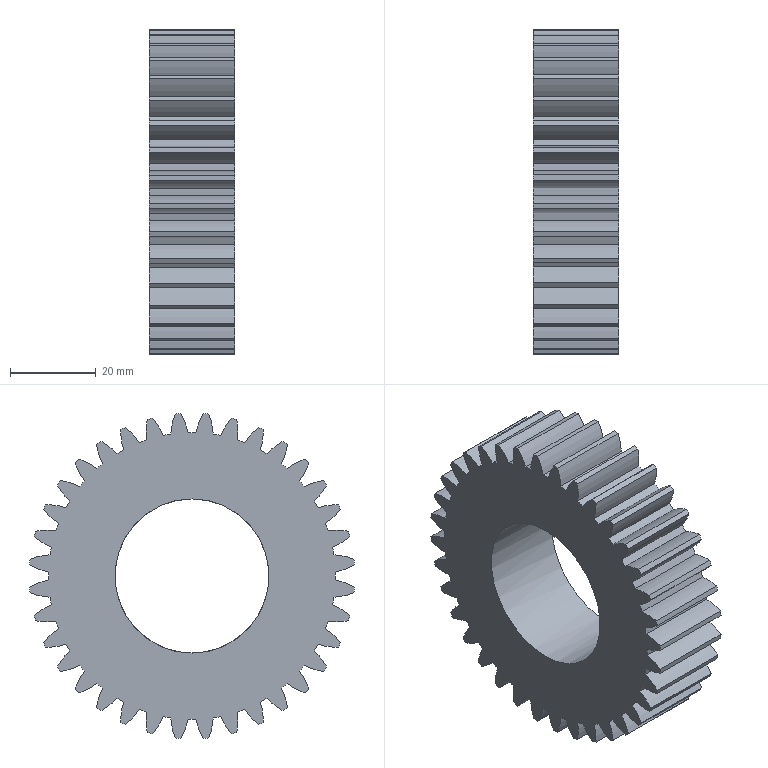Part | STEP file | spur gear_gb_GB - Spur gear 2M 36T 20PA 20FW ---S36A75H50L36.0N | 1 solid | 147 faces | box 20 x 75.809 x 75.809 mm | volume 59641 mm3 | cylinder 145 | plane 2 | commonest cylinder face diameters 28.8 x72 66.998 x36 76 x36 36 x1